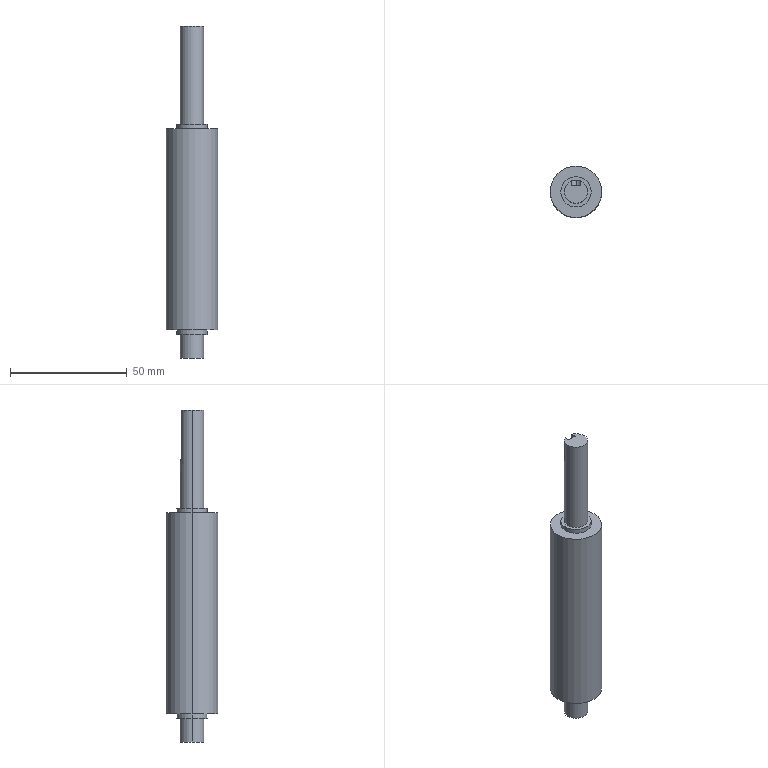Part | STEP file | 08-04 driving shaft | 1 solid | 21 faces | box 22 x 22 x 142 mm | volume 37102 mm3 | cylinder 12 | plane 9 | commonest cylinder face diameters 10 x4 13 x4 4 x2 22 x2
STEP:
#1=CARTESIAN_POINT('',(5.,0.,142.));
#2=VERTEX_POINT('',#1);
#3=CARTESIAN_POINT('',(2.,4.583,142.));
#4=VERTEX_POINT('',#3);
#5=CARTESIAN_POINT('',(0.,0.,142.));
#6=DIRECTION('',(0.,0.,1.));
#7=DIRECTION('',(1.,0.,0.));
#8=AXIS2_PLACEMENT_3D('',#5,#6,#7);
#9=CIRCLE('',#8,5.);
#10=EDGE_CURVE('',#2,#4,#9,.T.);
#11=ORIENTED_EDGE('',*,*,#10,.F.);
#12=CARTESIAN_POINT('',(5.,0.,100.));
#13=VERTEX_POINT('',#12);
#14=CARTESIAN_POINT('',(5.,0.,142.));
#15=DIRECTION('',(0.,0.,-1.));
#16=VECTOR('',#15,1000.);
#17=LINE('',#14,#16);
#18=EDGE_CURVE('',#2,#13,#17,.T.);
#19=ORIENTED_EDGE('',*,*,#18,.T.);
#20=CARTESIAN_POINT('',(-5.,0.,100.));
#21=VERTEX_POINT('',#20);
#22=CARTESIAN_POINT('',(0.,0.,100.));
#23=DIRECTION('',(0.,0.,1.));
#24=DIRECTION('',(1.,0.,0.));
#25=AXIS2_PLACEMENT_3D('',#22,#23,#24);
#26=CIRCLE('',#25,5.);
#27=EDGE_CURVE('',#13,#21,#26,.T.);
#28=ORIENTED_EDGE('',*,*,#27,.T.);
#29=CARTESIAN_POINT('',(-5.,0.,142.));
#30=VERTEX_POINT('',#29);
#31=CARTESIAN_POINT('',(-5.,0.,142.));
#32=DIRECTION('',(0.,0.,-1.));
#33=VECTOR('',#32,1000.);
#34=LINE('',#31,#33);
#35=EDGE_CURVE('',#30,#21,#34,.T.);
#36=ORIENTED_EDGE('',*,*,#35,.F.);
#37=CARTESIAN_POINT('',(-2.,4.583,142.));
#38=VERTEX_POINT('',#37);
#39=CARTESIAN_POINT('',(0.,0.,142.));
#40=DIRECTION('',(0.,0.,1.));
#41=DIRECTION('',(1.,0.,0.));
#42=AXIS2_PLACEMENT_3D('',#39,#40,#41);
#43=CIRCLE('',#42,5.);
#44=EDGE_CURVE('',#38,#30,#43,.T.);
#45=ORIENTED_EDGE('',*,*,#44,.F.);
#46=CARTESIAN_POINT('',(-2.,4.583,122.));
#47=VERTEX_POINT('',#46);
#48=CARTESIAN_POINT('',(-2.,4.583,142.));
#49=DIRECTION('',(0.,0.,-1.));
#50=VECTOR('',#49,1000.);
#51=LINE('',#48,#50);
#52=EDGE_CURVE('',#38,#47,#51,.T.);
#53=ORIENTED_EDGE('',*,*,#52,.T.);
#54=CARTESIAN_POINT('',(0.,5.,120.));
#55=VERTEX_POINT('',#54);
#56=CARTESIAN_POINT('',(-2.,4.583,122.));
#57=CARTESIAN_POINT('',(-2.,4.583,121.866));
#58=CARTESIAN_POINT('',(-1.987,4.588,121.735));
#59=CARTESIAN_POINT('',(-1.935,4.61,121.478));
#60=CARTESIAN_POINT('',(-1.896,4.627,121.35));
#61=CARTESIAN_POINT('',(-1.795,4.667,121.109));
#62=CARTESIAN_POINT('',(-1.734,4.69,120.995));
#63=CARTESIAN_POINT('',(-1.589,4.741,120.779));
#64=CARTESIAN_POINT('',(-1.506,4.769,120.678));
#65=CARTESIAN_POINT('',(-1.233,4.849,120.404));
#66=CARTESIAN_POINT('',(-1.012,4.903,120.255));
#67=CARTESIAN_POINT('',(-0.6519,4.959,120.105));
#68=CARTESIAN_POINT('',(-0.5246,4.974,120.066));
#69=CARTESIAN_POINT('',(-0.2652,4.995,120.013));
#70=CARTESIAN_POINT('',(-0.1336,5.,120.));
#71=CARTESIAN_POINT('',(0.,5.,120.));
#72=B_SPLINE_CURVE_WITH_KNOTS('',3,(#56,#57,#58,#59,#60,#61,#62,#63,#64,#65,#66,#67,#68,#69,#70,#71),.UNSPECIFIED.,.F.,.F.,(4,2,2,2,2,2,2,4),(0.,0.0003947,0.0007895,0.001184,0.001579,0.002368,0.002763,0.003158),.UNSPECIFIED.);
#73=EDGE_CURVE('',#47,#55,#72,.T.);
#74=ORIENTED_EDGE('',*,*,#73,.T.);
#75=CARTESIAN_POINT('',(2.,4.583,122.));
#76=VERTEX_POINT('',#75);
#77=CARTESIAN_POINT('',(0.,5.,120.));
#78=CARTESIAN_POINT('',(0.1336,5.,120.));
#79=CARTESIAN_POINT('',(0.2647,4.995,120.013));
#80=CARTESIAN_POINT('',(0.5221,4.974,120.065));
#81=CARTESIAN_POINT('',(0.6499,4.959,120.104));
#82=CARTESIAN_POINT('',(0.8914,4.921,120.205));
#83=CARTESIAN_POINT('',(1.006,4.899,120.266));
#84=CARTESIAN_POINT('',(1.222,4.85,120.411));
#85=CARTESIAN_POINT('',(1.323,4.823,120.495));
#86=CARTESIAN_POINT('',(1.597,4.742,120.768));
#87=CARTESIAN_POINT('',(1.745,4.687,120.989));
#88=CARTESIAN_POINT('',(1.895,4.627,121.348));
#89=CARTESIAN_POINT('',(1.935,4.611,121.475));
#90=CARTESIAN_POINT('',(1.987,4.588,121.735));
#91=CARTESIAN_POINT('',(2.,4.583,121.866));
#92=CARTESIAN_POINT('',(2.,4.583,122.));
#93=B_SPLINE_CURVE_WITH_KNOTS('',3,(#77,#78,#79,#80,#81,#82,#83,#84,#85,#86,#87,#88,#89,#90,#91,#92),.UNSPECIFIED.,.F.,.F.,(4,2,2,2,2,2,2,4),(0.,0.0003948,0.0007895,0.001184,0.001579,0.002369,0.002763,0.003158),.UNSPECIFIED.);
#94=EDGE_CURVE('',#55,#76,#93,.T.);
#95=ORIENTED_EDGE('',*,*,#94,.T.);
#96=CARTESIAN_POINT('',(2.,4.583,142.));
#97=DIRECTION('',(0.,0.,1.));
#98=VECTOR('',#97,1000.);
#99=LINE('',#96,#98);
#100=EDGE_CURVE('',#76,#4,#99,.T.);
#101=ORIENTED_EDGE('',*,*,#100,.T.);
#102=EDGE_LOOP('',(#11,#19,#28,#36,#45,#53,#74,#95,#101));
#103=FACE_OUTER_BOUND('',#102,.T.);
#104=CARTESIAN_POINT('',(0.,0.,142.));
#105=DIRECTION('',(0.,0.,-1.));
#106=DIRECTION('',(-1.,0.,0.));
#107=AXIS2_PLACEMENT_3D('',#104,#105,#106);
#108=CYLINDRICAL_SURFACE('',#107,5.);
#109=ADVANCED_FACE('',(#103),#108,.T.);
#110=CARTESIAN_POINT('',(6.5,0.,100.));
#111=VERTEX_POINT('',#110);
#112=CARTESIAN_POINT('',(-6.5,0.,100.));
#113=VERTEX_POINT('',#112);
#114=CARTESIAN_POINT('',(0.,0.,100.));
#115=DIRECTION('',(0.,0.,1.));
#116=DIRECTION('',(1.,0.,0.));
#117=AXIS2_PLACEMENT_3D('',#114,#115,#116);
#118=CIRCLE('',#117,6.5);
#119=EDGE_CURVE('',#111,#113,#118,.T.);
#120=ORIENTED_EDGE('',*,*,#119,.F.);
#121=CARTESIAN_POINT('',(6.5,0.,98.));
#122=VERTEX_POINT('',#121);
#123=CARTESIAN_POINT('',(6.5,0.,100.));
#124=DIRECTION('',(0.,0.,-1.));
#125=VECTOR('',#124,1000.);
#126=LINE('',#123,#125);
#127=EDGE_CURVE('',#111,#122,#126,.T.);
#128=ORIENTED_EDGE('',*,*,#127,.T.);
#129=CARTESIAN_POINT('',(-6.5,0.,98.));
#130=VERTEX_POINT('',#129);
#131=CARTESIAN_POINT('',(0.,0.,98.));
#132=DIRECTION('',(0.,0.,1.));
#133=DIRECTION('',(1.,0.,0.));
#134=AXIS2_PLACEMENT_3D('',#131,#132,#133);
#135=CIRCLE('',#134,6.5);
#136=EDGE_CURVE('',#122,#130,#135,.T.);
#137=ORIENTED_EDGE('',*,*,#136,.T.);
#138=CARTESIAN_POINT('',(-6.5,0.,100.));
#139=DIRECTION('',(0.,0.,-1.));
#140=VECTOR('',#139,1000.);
#141=LINE('',#138,#140);
#142=EDGE_CURVE('',#113,#130,#141,.T.);
#143=ORIENTED_EDGE('',*,*,#142,.F.);
#144=EDGE_LOOP('',(#120,#128,#137,#143));
#145=FACE_OUTER_BOUND('',#144,.T.);
#146=CARTESIAN_POINT('',(0.,0.,100.));
#147=DIRECTION('',(0.,0.,-1.));
#148=DIRECTION('',(-1.,0.,0.));
#149=AXIS2_PLACEMENT_3D('',#146,#147,#148);
#150=CYLINDRICAL_SURFACE('',#149,6.5);
#151=ADVANCED_FACE('',(#145),#150,.T.);
#152=CARTESIAN_POINT('',(-5.,0.,10.));
#153=VERTEX_POINT('',#152);
#154=CARTESIAN_POINT('',(5.,0.,10.));
#155=VERTEX_POINT('',#154);
#156=CARTESIAN_POINT('',(0.,0.,10.));
#157=DIRECTION('',(0.,0.,-1.));
#158=DIRECTION('',(-1.,0.,0.));
#159=AXIS2_PLACEMENT_3D('',#156,#157,#158);
#160=CIRCLE('',#159,5.);
#161=EDGE_CURVE('',#153,#155,#160,.T.);
#162=ORIENTED_EDGE('',*,*,#161,.T.);
#163=CARTESIAN_POINT('',(5.,0.,0.));
#164=VERTEX_POINT('',#163);
#165=CARTESIAN_POINT('',(5.,0.,12.));
#166=DIRECTION('',(0.,0.,-1.));
#167=VECTOR('',#166,1000.);
#168=LINE('',#165,#167);
#169=EDGE_CURVE('',#155,#164,#168,.T.);
#170=ORIENTED_EDGE('',*,*,#169,.T.);
#171=CARTESIAN_POINT('',(-5.,0.,0.));
#172=VERTEX_POINT('',#171);
#173=CARTESIAN_POINT('',(0.,0.,0.));
#174=DIRECTION('',(0.,0.,1.));
#175=DIRECTION('',(1.,0.,0.));
#176=AXIS2_PLACEMENT_3D('',#173,#174,#175);
#177=CIRCLE('',#176,5.);
#178=EDGE_CURVE('',#164,#172,#177,.T.);
#179=ORIENTED_EDGE('',*,*,#178,.T.);
#180=CARTESIAN_POINT('',(-5.,0.,12.));
#181=DIRECTION('',(0.,0.,-1.));
#182=VECTOR('',#181,1000.);
#183=LINE('',#180,#182);
#184=EDGE_CURVE('',#153,#172,#183,.T.);
#185=ORIENTED_EDGE('',*,*,#184,.F.);
#186=EDGE_LOOP('',(#162,#170,#179,#185));
#187=FACE_OUTER_BOUND('',#186,.T.);
#188=CARTESIAN_POINT('',(0.,0.,12.));
#189=DIRECTION('',(0.,0.,-1.));
#190=DIRECTION('',(-1.,0.,0.));
#191=AXIS2_PLACEMENT_3D('',#188,#189,#190);
#192=CYLINDRICAL_SURFACE('',#191,5.);
#193=ADVANCED_FACE('',(#187),#192,.T.);
#194=CARTESIAN_POINT('',(-6.5,0.,10.));
#195=VERTEX_POINT('',#194);
#196=CARTESIAN_POINT('',(6.5,0.,10.));
#197=VERTEX_POINT('',#196);
#198=CARTESIAN_POINT('',(0.,0.,10.));
#199=DIRECTION('',(0.,0.,-1.));
#200=DIRECTION('',(-1.,0.,0.));
#201=AXIS2_PLACEMENT_3D('',#198,#199,#200);
#202=CIRCLE('',#201,6.5);
#203=EDGE_CURVE('',#195,#197,#202,.T.);
#204=ORIENTED_EDGE('',*,*,#203,.F.);
#205=CARTESIAN_POINT('',(-6.5,0.,12.));
#206=VERTEX_POINT('',#205);
#207=CARTESIAN_POINT('',(-6.5,0.,10.));
#208=DIRECTION('',(0.,0.,1.));
#209=VECTOR('',#208,1000.);
#210=LINE('',#207,#209);
#211=EDGE_CURVE('',#195,#206,#210,.T.);
#212=ORIENTED_EDGE('',*,*,#211,.T.);
#213=CARTESIAN_POINT('',(6.5,0.,12.));
#214=VERTEX_POINT('',#213);
#215=CARTESIAN_POINT('',(0.,0.,12.));
#216=DIRECTION('',(0.,0.,-1.));
#217=DIRECTION('',(1.,0.,0.));
#218=AXIS2_PLACEMENT_3D('',#215,#216,#217);
#219=CIRCLE('',#218,6.5);
#220=EDGE_CURVE('',#206,#214,#219,.T.);
#221=ORIENTED_EDGE('',*,*,#220,.T.);
#222=CARTESIAN_POINT('',(6.5,0.,10.));
#223=DIRECTION('',(0.,0.,1.));
#224=VECTOR('',#223,1000.);
#225=LINE('',#222,#224);
#226=EDGE_CURVE('',#197,#214,#225,.T.);
#227=ORIENTED_EDGE('',*,*,#226,.F.);
#228=EDGE_LOOP('',(#204,#212,#221,#227));
#229=FACE_OUTER_BOUND('',#228,.T.);
#230=CARTESIAN_POINT('',(0.,0.,10.));
#231=DIRECTION('',(0.,0.,1.));
#232=DIRECTION('',(1.,0.,0.));
#233=AXIS2_PLACEMENT_3D('',#230,#231,#232);
#234=CYLINDRICAL_SURFACE('',#233,6.5);
#235=ADVANCED_FACE('',(#229),#234,.T.);
#236=CARTESIAN_POINT('',(11.,0.,98.));
#237=VERTEX_POINT('',#236);
#238=CARTESIAN_POINT('',(-11.,0.,98.));
#239=VERTEX_POINT('',#238);
#240=CARTESIAN_POINT('',(0.,0.,98.));
#241=DIRECTION('',(0.,0.,1.));
#242=DIRECTION('',(1.,0.,0.));
#243=AXIS2_PLACEMENT_3D('',#240,#241,#242);
#244=CIRCLE('',#243,11.);
#245=EDGE_CURVE('',#237,#239,#244,.T.);
#246=ORIENTED_EDGE('',*,*,#245,.F.);
#247=CARTESIAN_POINT('',(11.,0.,12.));
#248=VERTEX_POINT('',#247);
#249=CARTESIAN_POINT('',(11.,0.,98.));
#250=DIRECTION('',(0.,0.,-1.));
#251=VECTOR('',#250,1000.);
#252=LINE('',#249,#251);
#253=EDGE_CURVE('',#237,#248,#252,.T.);
#254=ORIENTED_EDGE('',*,*,#253,.T.);
#255=CARTESIAN_POINT('',(-11.,0.,12.));
#256=VERTEX_POINT('',#255);
#257=CARTESIAN_POINT('',(0.,0.,12.));
#258=DIRECTION('',(0.,0.,1.));
#259=DIRECTION('',(1.,0.,0.));
#260=AXIS2_PLACEMENT_3D('',#257,#258,#259);
#261=CIRCLE('',#260,11.);
#262=EDGE_CURVE('',#248,#256,#261,.T.);
#263=ORIENTED_EDGE('',*,*,#262,.T.);
#264=CARTESIAN_POINT('',(-11.,0.,98.));
#265=DIRECTION('',(0.,0.,-1.));
#266=VECTOR('',#265,1000.);
#267=LINE('',#264,#266);
#268=EDGE_CURVE('',#239,#256,#267,.T.);
#269=ORIENTED_EDGE('',*,*,#268,.F.);
#270=EDGE_LOOP('',(#246,#254,#263,#269));
#271=FACE_OUTER_BOUND('',#270,.T.);
#272=CARTESIAN_POINT('',(0.,0.,98.));
#273=DIRECTION('',(0.,0.,-1.));
#274=DIRECTION('',(-1.,0.,0.));
#275=AXIS2_PLACEMENT_3D('',#272,#273,#274);
#276=CYLINDRICAL_SURFACE('',#275,11.);
#277=ADVANCED_FACE('',(#271),#276,.T.);
#278=CARTESIAN_POINT('',(0.,0.,100.));
#279=DIRECTION('',(0.,0.,1.));
#280=DIRECTION('',(1.,0.,0.));
#281=AXIS2_PLACEMENT_3D('',#278,#279,#280);
#282=CIRCLE('',#281,6.5);
#283=EDGE_CURVE('',#113,#111,#282,.T.);
#284=ORIENTED_EDGE('',*,*,#283,.T.);
#285=ORIENTED_EDGE('',*,*,#119,.T.);
#286=EDGE_LOOP('',(#284,#285));
#287=FACE_OUTER_BOUND('',#286,.T.);
#288=CARTESIAN_POINT('',(0.,0.,100.));
#289=DIRECTION('',(0.,0.,1.));
#290=DIRECTION('',(1.,0.,0.));
#291=AXIS2_PLACEMENT_3D('',#288,#289,#290);
#292=CIRCLE('',#291,5.);
#293=EDGE_CURVE('',#21,#13,#292,.T.);
#294=ORIENTED_EDGE('',*,*,#293,.F.);
#295=ORIENTED_EDGE('',*,*,#27,.F.);
#296=EDGE_LOOP('',(#294,#295));
#297=FACE_BOUND('',#296,.T.);
#298=CARTESIAN_POINT('',(0.,0.,100.));
#299=DIRECTION('',(0.,0.,1.));
#300=DIRECTION('',(1.,0.,0.));
#301=AXIS2_PLACEMENT_3D('',#298,#299,#300);
#302=PLANE('',#301);
#303=ADVANCED_FACE('',(#287,#297),#302,.T.);
#304=CARTESIAN_POINT('',(0.,0.,98.));
#305=DIRECTION('',(0.,0.,1.));
#306=DIRECTION('',(1.,0.,0.));
#307=AXIS2_PLACEMENT_3D('',#304,#305,#306);
#308=CIRCLE('',#307,11.);
#309=EDGE_CURVE('',#239,#237,#308,.T.);
#310=ORIENTED_EDGE('',*,*,#309,.T.);
#311=ORIENTED_EDGE('',*,*,#245,.T.);
#312=EDGE_LOOP('',(#310,#311));
#313=FACE_OUTER_BOUND('',#312,.T.);
#314=CARTESIAN_POINT('',(0.,0.,98.));
#315=DIRECTION('',(0.,0.,1.));
#316=DIRECTION('',(1.,0.,0.));
#317=AXIS2_PLACEMENT_3D('',#314,#315,#316);
#318=CIRCLE('',#317,6.5);
#319=EDGE_CURVE('',#130,#122,#318,.T.);
#320=ORIENTED_EDGE('',*,*,#319,.F.);
#321=ORIENTED_EDGE('',*,*,#136,.F.);
#322=EDGE_LOOP('',(#320,#321));
#323=FACE_BOUND('',#322,.T.);
#324=CARTESIAN_POINT('',(0.,0.,98.));
#325=DIRECTION('',(0.,0.,1.));
#326=DIRECTION('',(1.,0.,0.));
#327=AXIS2_PLACEMENT_3D('',#324,#325,#326);
#328=PLANE('',#327);
#329=ADVANCED_FACE('',(#313,#323),#328,.T.);
#330=CARTESIAN_POINT('',(0.,0.,12.));
#331=DIRECTION('',(0.,0.,1.));
#332=DIRECTION('',(1.,0.,0.));
#333=AXIS2_PLACEMENT_3D('',#330,#331,#332);
#334=CIRCLE('',#333,11.);
#335=EDGE_CURVE('',#256,#248,#334,.T.);
#336=ORIENTED_EDGE('',*,*,#335,.F.);
#337=ORIENTED_EDGE('',*,*,#262,.F.);
#338=EDGE_LOOP('',(#336,#337));
#339=FACE_OUTER_BOUND('',#338,.T.);
#340=CARTESIAN_POINT('',(0.,0.,12.));
#341=DIRECTION('',(0.,0.,-1.));
#342=DIRECTION('',(1.,0.,0.));
#343=AXIS2_PLACEMENT_3D('',#340,#341,#342);
#344=CIRCLE('',#343,6.5);
#345=EDGE_CURVE('',#214,#206,#344,.T.);
#346=ORIENTED_EDGE('',*,*,#345,.F.);
#347=ORIENTED_EDGE('',*,*,#220,.F.);
#348=EDGE_LOOP('',(#346,#347));
#349=FACE_BOUND('',#348,.T.);
#350=CARTESIAN_POINT('',(0.,0.,12.));
#351=DIRECTION('',(0.,0.,1.));
#352=DIRECTION('',(1.,0.,0.));
#353=AXIS2_PLACEMENT_3D('',#350,#351,#352);
#354=PLANE('',#353);
#355=ADVANCED_FACE('',(#339,#349),#354,.F.);
#356=ORIENTED_EDGE('',*,*,#253,.F.);
#357=ORIENTED_EDGE('',*,*,#309,.F.);
#358=ORIENTED_EDGE('',*,*,#268,.T.);
#359=ORIENTED_EDGE('',*,*,#335,.T.);
#360=EDGE_LOOP('',(#356,#357,#358,#359));
#361=FACE_OUTER_BOUND('',#360,.T.);
#362=CARTESIAN_POINT('',(0.,0.,98.));
#363=DIRECTION('',(0.,0.,-1.));
#364=DIRECTION('',(-1.,0.,0.));
#365=AXIS2_PLACEMENT_3D('',#362,#363,#364);
#366=CYLINDRICAL_SURFACE('',#365,11.);
#367=ADVANCED_FACE('',(#361),#366,.T.);
#368=CARTESIAN_POINT('',(0.,0.,10.));
#369=DIRECTION('',(0.,0.,-1.));
#370=DIRECTION('',(-1.,0.,0.));
#371=AXIS2_PLACEMENT_3D('',#368,#369,#370);
#372=CIRCLE('',#371,6.5);
#373=EDGE_CURVE('',#197,#195,#372,.T.);
#374=ORIENTED_EDGE('',*,*,#373,.T.);
#375=ORIENTED_EDGE('',*,*,#203,.T.);
#376=EDGE_LOOP('',(#374,#375));
#377=FACE_OUTER_BOUND('',#376,.T.);
#378=ORIENTED_EDGE('',*,*,#161,.F.);
#379=CARTESIAN_POINT('',(0.,0.,10.));
#380=DIRECTION('',(0.,0.,-1.));
#381=DIRECTION('',(-1.,0.,0.));
#382=AXIS2_PLACEMENT_3D('',#379,#380,#381);
#383=CIRCLE('',#382,5.);
#384=EDGE_CURVE('',#155,#153,#383,.T.);
#385=ORIENTED_EDGE('',*,*,#384,.F.);
#386=EDGE_LOOP('',(#378,#385));
#387=FACE_BOUND('',#386,.T.);
#388=CARTESIAN_POINT('',(0.,0.,10.));
#389=DIRECTION('',(0.,0.,-1.));
#390=DIRECTION('',(-1.,0.,0.));
#391=AXIS2_PLACEMENT_3D('',#388,#389,#390);
#392=PLANE('',#391);
#393=ADVANCED_FACE('',(#377,#387),#392,.T.);
#394=ORIENTED_EDGE('',*,*,#211,.F.);
#395=ORIENTED_EDGE('',*,*,#373,.F.);
#396=ORIENTED_EDGE('',*,*,#226,.T.);
#397=ORIENTED_EDGE('',*,*,#345,.T.);
#398=EDGE_LOOP('',(#394,#395,#396,#397));
#399=FACE_OUTER_BOUND('',#398,.T.);
#400=CARTESIAN_POINT('',(0.,0.,10.));
#401=DIRECTION('',(0.,0.,1.));
#402=DIRECTION('',(1.,0.,0.));
#403=AXIS2_PLACEMENT_3D('',#400,#401,#402);
#404=CYLINDRICAL_SURFACE('',#403,6.5);
#405=ADVANCED_FACE('',(#399),#404,.T.);
#406=CARTESIAN_POINT('',(0.,0.,0.));
#407=DIRECTION('',(0.,0.,1.));
#408=DIRECTION('',(1.,0.,0.));
#409=AXIS2_PLACEMENT_3D('',#406,#407,#408);
#410=CIRCLE('',#409,5.);
#411=EDGE_CURVE('',#172,#164,#410,.T.);
#412=ORIENTED_EDGE('',*,*,#411,.F.);
#413=ORIENTED_EDGE('',*,*,#178,.F.);
#414=EDGE_LOOP('',(#412,#413));
#415=FACE_OUTER_BOUND('',#414,.T.);
#416=CARTESIAN_POINT('',(0.,0.,0.));
#417=DIRECTION('',(0.,0.,1.));
#418=DIRECTION('',(1.,0.,0.));
#419=AXIS2_PLACEMENT_3D('',#416,#417,#418);
#420=PLANE('',#419);
#421=ADVANCED_FACE('',(#415),#420,.F.);
#422=ORIENTED_EDGE('',*,*,#169,.F.);
#423=ORIENTED_EDGE('',*,*,#384,.T.);
#424=ORIENTED_EDGE('',*,*,#184,.T.);
#425=ORIENTED_EDGE('',*,*,#411,.T.);
#426=EDGE_LOOP('',(#422,#423,#424,#425));
#427=FACE_OUTER_BOUND('',#426,.T.);
#428=CARTESIAN_POINT('',(0.,0.,12.));
#429=DIRECTION('',(0.,0.,-1.));
#430=DIRECTION('',(-1.,0.,0.));
#431=AXIS2_PLACEMENT_3D('',#428,#429,#430);
#432=CYLINDRICAL_SURFACE('',#431,5.);
#433=ADVANCED_FACE('',(#427),#432,.T.);
#434=ORIENTED_EDGE('',*,*,#127,.F.);
#435=ORIENTED_EDGE('',*,*,#283,.F.);
#436=ORIENTED_EDGE('',*,*,#142,.T.);
#437=ORIENTED_EDGE('',*,*,#319,.T.);
#438=EDGE_LOOP('',(#434,#435,#436,#437));
#439=FACE_OUTER_BOUND('',#438,.T.);
#440=CARTESIAN_POINT('',(0.,0.,100.));
#441=DIRECTION('',(0.,0.,-1.));
#442=DIRECTION('',(-1.,0.,0.));
#443=AXIS2_PLACEMENT_3D('',#440,#441,#442);
#444=CYLINDRICAL_SURFACE('',#443,6.5);
#445=ADVANCED_FACE('',(#439),#444,.T.);
#446=CARTESIAN_POINT('',(2.,2.5,122.));
#447=VERTEX_POINT('',#446);
#448=CARTESIAN_POINT('',(0.,2.5,120.));
#449=VERTEX_POINT('',#448);
#450=CARTESIAN_POINT('',(0.,2.5,122.));
#451=DIRECTION('',(0.,1.,0.));
#452=DIRECTION('',(0.,0.,-1.));
#453=AXIS2_PLACEMENT_3D('',#450,#451,#452);
#454=CIRCLE('',#453,2.);
#455=EDGE_CURVE('',#447,#449,#454,.T.);
#456=ORIENTED_EDGE('',*,*,#455,.T.);
#457=CARTESIAN_POINT('',(-2.,2.5,122.));
#458=VERTEX_POINT('',#457);
#459=CARTESIAN_POINT('',(0.,2.5,122.));
#460=DIRECTION('',(0.,1.,0.));
#461=DIRECTION('',(0.,0.,-1.));
#462=AXIS2_PLACEMENT_3D('',#459,#460,#461);
#463=CIRCLE('',#462,2.);
#464=EDGE_CURVE('',#449,#458,#463,.T.);
#465=ORIENTED_EDGE('',*,*,#464,.T.);
#466=CARTESIAN_POINT('',(-2.,2.5,142.));
#467=VERTEX_POINT('',#466);
#468=CARTESIAN_POINT('',(-2.,2.5,115.056));
#469=DIRECTION('',(0.,0.,1.));
#470=VECTOR('',#469,1000.);
#471=LINE('',#468,#470);
#472=EDGE_CURVE('',#458,#467,#471,.T.);
#473=ORIENTED_EDGE('',*,*,#472,.T.);
#474=CARTESIAN_POINT('',(2.,2.5,142.));
#475=VERTEX_POINT('',#474);
#476=CARTESIAN_POINT('',(-2.,2.5,142.));
#477=DIRECTION('',(1.,0.,0.));
#478=VECTOR('',#477,1000.);
#479=LINE('',#476,#478);
#480=EDGE_CURVE('',#467,#475,#479,.T.);
#481=ORIENTED_EDGE('',*,*,#480,.T.);
#482=CARTESIAN_POINT('',(2.,2.5,115.056));
#483=DIRECTION('',(0.,0.,1.));
#484=VECTOR('',#483,1000.);
#485=LINE('',#482,#484);
#486=EDGE_CURVE('',#447,#475,#485,.T.);
#487=ORIENTED_EDGE('',*,*,#486,.F.);
#488=EDGE_LOOP('',(#456,#465,#473,#481,#487));
#489=FACE_OUTER_BOUND('',#488,.T.);
#490=CARTESIAN_POINT('',(-2.,2.5,115.056));
#491=DIRECTION('',(0.,-1.,0.));
#492=DIRECTION('',(0.,0.,-1.));
#493=AXIS2_PLACEMENT_3D('',#490,#491,#492);
#494=PLANE('',#493);
#495=ADVANCED_FACE('',(#489),#494,.F.);
#496=CARTESIAN_POINT('',(-2.,0.,142.));
#497=DIRECTION('',(0.,-1.,0.));
#498=VECTOR('',#497,1000.);
#499=LINE('',#496,#498);
#500=EDGE_CURVE('',#38,#467,#499,.T.);
#501=ORIENTED_EDGE('',*,*,#500,.F.);
#502=ORIENTED_EDGE('',*,*,#44,.T.);
#503=CARTESIAN_POINT('',(0.,0.,142.));
#504=DIRECTION('',(0.,0.,1.));
#505=DIRECTION('',(1.,0.,0.));
#506=AXIS2_PLACEMENT_3D('',#503,#504,#505);
#507=CIRCLE('',#506,5.);
#508=EDGE_CURVE('',#30,#2,#507,.T.);
#509=ORIENTED_EDGE('',*,*,#508,.T.);
#510=ORIENTED_EDGE('',*,*,#10,.T.);
#511=CARTESIAN_POINT('',(2.,5.405,142.));
#512=DIRECTION('',(0.,1.,0.));
#513=VECTOR('',#512,1000.);
#514=LINE('',#511,#513);
#515=EDGE_CURVE('',#475,#4,#514,.T.);
#516=ORIENTED_EDGE('',*,*,#515,.F.);
#517=ORIENTED_EDGE('',*,*,#480,.F.);
#518=EDGE_LOOP('',(#501,#502,#509,#510,#516,#517));
#519=FACE_OUTER_BOUND('',#518,.T.);
#520=CARTESIAN_POINT('',(0.,0.,142.));
#521=DIRECTION('',(0.,0.,1.));
#522=DIRECTION('',(1.,0.,0.));
#523=AXIS2_PLACEMENT_3D('',#520,#521,#522);
#524=PLANE('',#523);
#525=ADVANCED_FACE('',(#519),#524,.T.);
#526=ORIENTED_EDGE('',*,*,#100,.F.);
#527=CARTESIAN_POINT('',(2.,5.405,122.));
#528=DIRECTION('',(0.,-1.,0.));
#529=VECTOR('',#528,1000.);
#530=LINE('',#527,#529);
#531=EDGE_CURVE('',#76,#447,#530,.T.);
#532=ORIENTED_EDGE('',*,*,#531,.T.);
#533=ORIENTED_EDGE('',*,*,#486,.T.);
#534=ORIENTED_EDGE('',*,*,#515,.T.);
#535=EDGE_LOOP('',(#526,#532,#533,#534));
#536=FACE_OUTER_BOUND('',#535,.T.);
#537=CARTESIAN_POINT('',(2.,5.405,115.056));
#538=DIRECTION('',(1.,0.,0.));
#539=DIRECTION('',(0.,1.,0.));
#540=AXIS2_PLACEMENT_3D('',#537,#538,#539);
#541=PLANE('',#540);
#542=ADVANCED_FACE('',(#536),#541,.F.);
#543=CARTESIAN_POINT('',(0.,0.,120.));
#544=DIRECTION('',(0.,1.,0.));
#545=VECTOR('',#544,1000.);
#546=LINE('',#543,#545);
#547=EDGE_CURVE('',#449,#55,#546,.T.);
#548=ORIENTED_EDGE('',*,*,#547,.F.);
#549=ORIENTED_EDGE('',*,*,#455,.F.);
#550=ORIENTED_EDGE('',*,*,#531,.F.);
#551=ORIENTED_EDGE('',*,*,#94,.F.);
#552=EDGE_LOOP('',(#548,#549,#550,#551));
#553=FACE_OUTER_BOUND('',#552,.T.);
#554=CARTESIAN_POINT('',(0.,5.405,122.));
#555=DIRECTION('',(0.,-1.,0.));
#556=DIRECTION('',(1.,0.,0.));
#557=AXIS2_PLACEMENT_3D('',#554,#555,#556);
#558=CYLINDRICAL_SURFACE('',#557,2.);
#559=ADVANCED_FACE('',(#553),#558,.F.);
#560=ORIENTED_EDGE('',*,*,#464,.F.);
#561=ORIENTED_EDGE('',*,*,#547,.T.);
#562=ORIENTED_EDGE('',*,*,#73,.F.);
#563=CARTESIAN_POINT('',(-2.,5.405,122.));
#564=DIRECTION('',(0.,1.,0.));
#565=VECTOR('',#564,1000.);
#566=LINE('',#563,#565);
#567=EDGE_CURVE('',#458,#47,#566,.T.);
#568=ORIENTED_EDGE('',*,*,#567,.F.);
#569=EDGE_LOOP('',(#560,#561,#562,#568));
#570=FACE_OUTER_BOUND('',#569,.T.);
#571=CARTESIAN_POINT('',(0.,5.405,122.));
#572=DIRECTION('',(0.,1.,0.));
#573=DIRECTION('',(-1.,0.,0.));
#574=AXIS2_PLACEMENT_3D('',#571,#572,#573);
#575=CYLINDRICAL_SURFACE('',#574,2.);
#576=ADVANCED_FACE('',(#570),#575,.F.);
#577=ORIENTED_EDGE('',*,*,#472,.F.);
#578=ORIENTED_EDGE('',*,*,#567,.T.);
#579=ORIENTED_EDGE('',*,*,#52,.F.);
#580=ORIENTED_EDGE('',*,*,#500,.T.);
#581=EDGE_LOOP('',(#577,#578,#579,#580));
#582=FACE_OUTER_BOUND('',#581,.T.);
#583=CARTESIAN_POINT('',(-2.,5.405,115.056));
#584=DIRECTION('',(-1.,0.,0.));
#585=DIRECTION('',(0.,-1.,0.));
#586=AXIS2_PLACEMENT_3D('',#583,#584,#585);
#587=PLANE('',#586);
#588=ADVANCED_FACE('',(#582),#587,.F.);
#589=ORIENTED_EDGE('',*,*,#18,.F.);
#590=ORIENTED_EDGE('',*,*,#508,.F.);
#591=ORIENTED_EDGE('',*,*,#35,.T.);
#592=ORIENTED_EDGE('',*,*,#293,.T.);
#593=EDGE_LOOP('',(#589,#590,#591,#592));
#594=FACE_OUTER_BOUND('',#593,.T.);
#595=CARTESIAN_POINT('',(0.,0.,142.));
#596=DIRECTION('',(0.,0.,-1.));
#597=DIRECTION('',(-1.,0.,0.));
#598=AXIS2_PLACEMENT_3D('',#595,#596,#597);
#599=CYLINDRICAL_SURFACE('',#598,5.);
#600=ADVANCED_FACE('',(#594),#599,.T.);
#601=CLOSED_SHELL('',(#109,#151,#193,#235,#277,#303,#329,#355,#367,#393,#405,#421,#433,#445,#495,#525,#542,#559,#576,#588,#600));
#602=MANIFOLD_SOLID_BREP('',#601);
#603=CARTESIAN_POINT('',(0.,0.,0.));
#604=DIRECTION('',(0.,0.,1.));
#605=DIRECTION('',(1.,0.,0.));
#606=AXIS2_PLACEMENT_3D('',#603,#604,#605);
#607=(LENGTH_UNIT()NAMED_UNIT(*)SI_UNIT(.MILLI.,.METRE.));
#608=UNCERTAINTY_MEASURE_WITH_UNIT(LENGTH_MEASURE(0.00001),#607,'','');
#609=(NAMED_UNIT(*)PLANE_ANGLE_UNIT()SI_UNIT($,.RADIAN.));
#610=(NAMED_UNIT(*)SI_UNIT($,.STERADIAN.)SOLID_ANGLE_UNIT());
#611=(GEOMETRIC_REPRESENTATION_CONTEXT(3)GLOBAL_UNCERTAINTY_ASSIGNED_CONTEXT((#608))GLOBAL_UNIT_ASSIGNED_CONTEXT((#607,#609,#610))REPRESENTATION_CONTEXT('',''));
#612=ADVANCED_BREP_SHAPE_REPRESENTATION('',(#602,#606),#611);